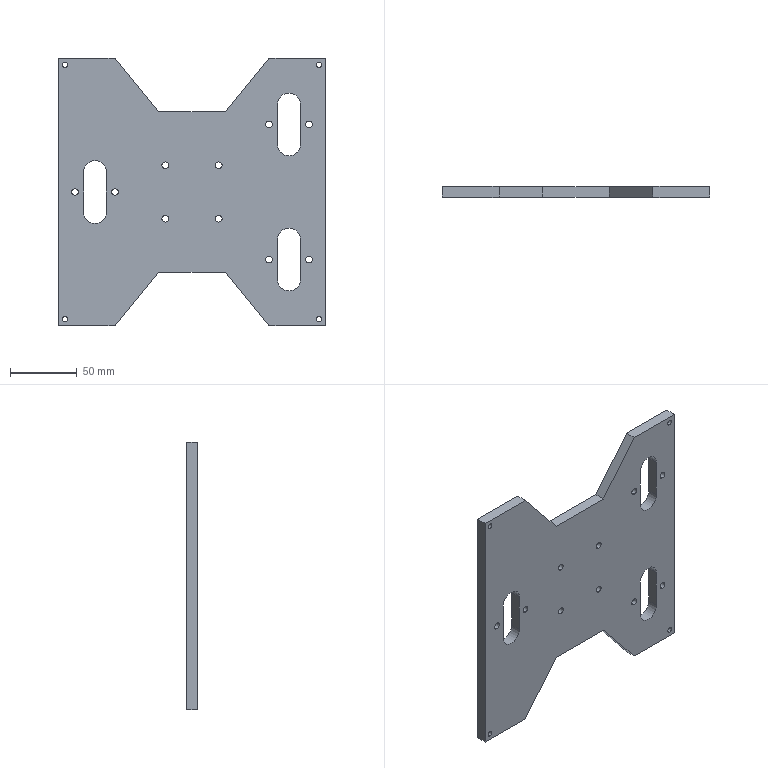Part | SolidWorks | features Cut 1, Extrusion 1, ICE 1 | 1 solid | 57 faces | box 200 x 8 x 200 mm | volume 247540 mm3 | cylinder 37 | plane 20 | commonest cylinder face diameters 5 x20 17 x9 4 x8